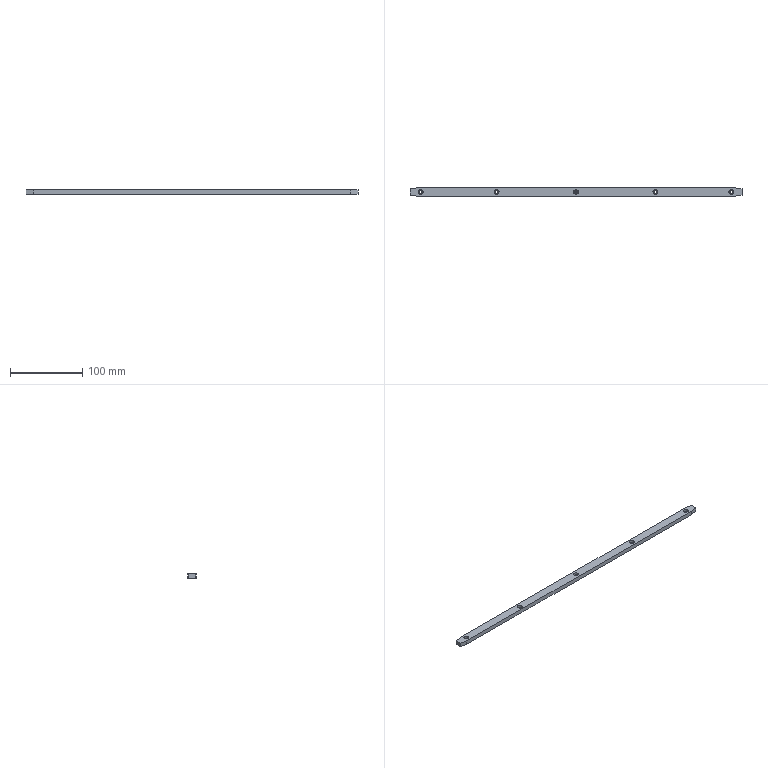Part | NX | features BREP 1 | 1 solid | 35 faces | box 460 x 12 x 6 mm | volume 32178 mm3 | cylinder 20 | plane 15 | commonest cylinder face diameters 3.4 x10 6.7 x10
STEP:
#1=CARTESIAN_POINT('',(-113.35,0.,-0.5));
#2=VERTEX_POINT('',#1);
#3=CARTESIAN_POINT('',(-106.65,0.,-0.5));
#4=VERTEX_POINT('',#3);
#5=CARTESIAN_POINT('',(-110.,0.,-0.5));
#6=DIRECTION('',(0.,0.,1.));
#7=DIRECTION('',(1.,0.,0.));
#8=AXIS2_PLACEMENT_3D('',#5,#6,#7);
#9=CIRCLE('',#8,3.35);
#10=EDGE_CURVE('',#2,#4,#9,.T.);
#11=ORIENTED_EDGE('',*,*,#10,.F.);
#12=CARTESIAN_POINT('',(-113.35,0.,3.));
#13=VERTEX_POINT('',#12);
#14=CARTESIAN_POINT('',(-113.35,0.,3.));
#15=DIRECTION('',(0.,0.,1.));
#16=VECTOR('',#15,1000.);
#17=LINE('',#14,#16);
#18=EDGE_CURVE('',#13,#2,#17,.F.);
#19=ORIENTED_EDGE('',*,*,#18,.F.);
#20=CARTESIAN_POINT('',(-106.65,0.,3.));
#21=VERTEX_POINT('',#20);
#22=CARTESIAN_POINT('',(-110.,0.,3.));
#23=DIRECTION('',(0.,0.,1.));
#24=DIRECTION('',(1.,0.,0.));
#25=AXIS2_PLACEMENT_3D('',#22,#23,#24);
#26=CIRCLE('',#25,3.35);
#27=EDGE_CURVE('',#13,#21,#26,.T.);
#28=ORIENTED_EDGE('',*,*,#27,.T.);
#29=CARTESIAN_POINT('',(-106.65,0.,3.));
#30=DIRECTION('',(0.,0.,1.));
#31=VECTOR('',#30,1000.);
#32=LINE('',#29,#31);
#33=EDGE_CURVE('',#21,#4,#32,.F.);
#34=ORIENTED_EDGE('',*,*,#33,.T.);
#35=EDGE_LOOP('',(#11,#19,#28,#34));
#36=FACE_BOUND('',#35,.T.);
#37=CARTESIAN_POINT('',(-110.,0.,3.));
#38=DIRECTION('',(0.,0.,1.));
#39=DIRECTION('',(1.,0.,0.));
#40=AXIS2_PLACEMENT_3D('',#37,#38,#39);
#41=CYLINDRICAL_SURFACE('',#40,3.35);
#42=ADVANCED_FACE('',(#36),#41,.F.);
#43=CARTESIAN_POINT('',(-111.7,0.,-3.));
#44=VERTEX_POINT('',#43);
#45=CARTESIAN_POINT('',(-108.3,0.,-3.));
#46=VERTEX_POINT('',#45);
#47=CARTESIAN_POINT('',(-110.,0.,-3.));
#48=DIRECTION('',(0.,0.,1.));
#49=DIRECTION('',(1.,0.,0.));
#50=AXIS2_PLACEMENT_3D('',#47,#48,#49);
#51=CIRCLE('',#50,1.7);
#52=EDGE_CURVE('',#44,#46,#51,.T.);
#53=ORIENTED_EDGE('',*,*,#52,.F.);
#54=CARTESIAN_POINT('',(-111.7,0.,-0.5));
#55=VERTEX_POINT('',#54);
#56=CARTESIAN_POINT('',(-111.7,0.,3.));
#57=DIRECTION('',(0.,0.,1.));
#58=VECTOR('',#57,1000.);
#59=LINE('',#56,#58);
#60=EDGE_CURVE('',#55,#44,#59,.F.);
#61=ORIENTED_EDGE('',*,*,#60,.F.);
#62=CARTESIAN_POINT('',(-108.3,0.,-0.5));
#63=VERTEX_POINT('',#62);
#64=CARTESIAN_POINT('',(-110.,0.,-0.5));
#65=DIRECTION('',(0.,0.,1.));
#66=DIRECTION('',(1.,0.,0.));
#67=AXIS2_PLACEMENT_3D('',#64,#65,#66);
#68=CIRCLE('',#67,1.7);
#69=EDGE_CURVE('',#55,#63,#68,.T.);
#70=ORIENTED_EDGE('',*,*,#69,.T.);
#71=CARTESIAN_POINT('',(-108.3,0.,3.));
#72=DIRECTION('',(0.,0.,1.));
#73=VECTOR('',#72,1000.);
#74=LINE('',#71,#73);
#75=EDGE_CURVE('',#63,#46,#74,.F.);
#76=ORIENTED_EDGE('',*,*,#75,.T.);
#77=EDGE_LOOP('',(#53,#61,#70,#76));
#78=FACE_BOUND('',#77,.T.);
#79=CARTESIAN_POINT('',(-110.,0.,3.));
#80=DIRECTION('',(0.,0.,1.));
#81=DIRECTION('',(1.,0.,0.));
#82=AXIS2_PLACEMENT_3D('',#79,#80,#81);
#83=CYLINDRICAL_SURFACE('',#82,1.7);
#84=ADVANCED_FACE('',(#78),#83,.F.);
#85=CARTESIAN_POINT('',(106.65,0.,-0.5));
#86=VERTEX_POINT('',#85);
#87=CARTESIAN_POINT('',(113.35,0.,-0.5));
#88=VERTEX_POINT('',#87);
#89=CARTESIAN_POINT('',(110.,0.,-0.5));
#90=DIRECTION('',(0.,0.,1.));
#91=DIRECTION('',(1.,0.,0.));
#92=AXIS2_PLACEMENT_3D('',#89,#90,#91);
#93=CIRCLE('',#92,3.35);
#94=EDGE_CURVE('',#86,#88,#93,.T.);
#95=ORIENTED_EDGE('',*,*,#94,.F.);
#96=CARTESIAN_POINT('',(106.65,0.,3.));
#97=VERTEX_POINT('',#96);
#98=CARTESIAN_POINT('',(106.65,0.,3.));
#99=DIRECTION('',(0.,0.,1.));
#100=VECTOR('',#99,1000.);
#101=LINE('',#98,#100);
#102=EDGE_CURVE('',#97,#86,#101,.F.);
#103=ORIENTED_EDGE('',*,*,#102,.F.);
#104=CARTESIAN_POINT('',(113.35,0.,3.));
#105=VERTEX_POINT('',#104);
#106=CARTESIAN_POINT('',(110.,0.,3.));
#107=DIRECTION('',(0.,0.,1.));
#108=DIRECTION('',(1.,0.,0.));
#109=AXIS2_PLACEMENT_3D('',#106,#107,#108);
#110=CIRCLE('',#109,3.35);
#111=EDGE_CURVE('',#97,#105,#110,.T.);
#112=ORIENTED_EDGE('',*,*,#111,.T.);
#113=CARTESIAN_POINT('',(113.35,0.,3.));
#114=DIRECTION('',(0.,0.,1.));
#115=VECTOR('',#114,1000.);
#116=LINE('',#113,#115);
#117=EDGE_CURVE('',#105,#88,#116,.F.);
#118=ORIENTED_EDGE('',*,*,#117,.T.);
#119=EDGE_LOOP('',(#95,#103,#112,#118));
#120=FACE_BOUND('',#119,.T.);
#121=CARTESIAN_POINT('',(110.,0.,3.));
#122=DIRECTION('',(0.,0.,1.));
#123=DIRECTION('',(1.,0.,0.));
#124=AXIS2_PLACEMENT_3D('',#121,#122,#123);
#125=CYLINDRICAL_SURFACE('',#124,3.35);
#126=ADVANCED_FACE('',(#120),#125,.F.);
#127=CARTESIAN_POINT('',(108.3,0.,-3.));
#128=VERTEX_POINT('',#127);
#129=CARTESIAN_POINT('',(111.7,0.,-3.));
#130=VERTEX_POINT('',#129);
#131=CARTESIAN_POINT('',(110.,0.,-3.));
#132=DIRECTION('',(0.,0.,1.));
#133=DIRECTION('',(1.,0.,0.));
#134=AXIS2_PLACEMENT_3D('',#131,#132,#133);
#135=CIRCLE('',#134,1.7);
#136=EDGE_CURVE('',#128,#130,#135,.T.);
#137=ORIENTED_EDGE('',*,*,#136,.F.);
#138=CARTESIAN_POINT('',(108.3,0.,-0.5));
#139=VERTEX_POINT('',#138);
#140=CARTESIAN_POINT('',(108.3,0.,3.));
#141=DIRECTION('',(0.,0.,1.));
#142=VECTOR('',#141,1000.);
#143=LINE('',#140,#142);
#144=EDGE_CURVE('',#139,#128,#143,.F.);
#145=ORIENTED_EDGE('',*,*,#144,.F.);
#146=CARTESIAN_POINT('',(111.7,0.,-0.5));
#147=VERTEX_POINT('',#146);
#148=CARTESIAN_POINT('',(110.,0.,-0.5));
#149=DIRECTION('',(0.,0.,1.));
#150=DIRECTION('',(1.,0.,0.));
#151=AXIS2_PLACEMENT_3D('',#148,#149,#150);
#152=CIRCLE('',#151,1.7);
#153=EDGE_CURVE('',#139,#147,#152,.T.);
#154=ORIENTED_EDGE('',*,*,#153,.T.);
#155=CARTESIAN_POINT('',(111.7,0.,3.));
#156=DIRECTION('',(0.,0.,1.));
#157=VECTOR('',#156,1000.);
#158=LINE('',#155,#157);
#159=EDGE_CURVE('',#147,#130,#158,.F.);
#160=ORIENTED_EDGE('',*,*,#159,.T.);
#161=EDGE_LOOP('',(#137,#145,#154,#160));
#162=FACE_BOUND('',#161,.T.);
#163=CARTESIAN_POINT('',(110.,0.,3.));
#164=DIRECTION('',(0.,0.,1.));
#165=DIRECTION('',(1.,0.,0.));
#166=AXIS2_PLACEMENT_3D('',#163,#164,#165);
#167=CYLINDRICAL_SURFACE('',#166,1.7);
#168=ADVANCED_FACE('',(#162),#167,.F.);
#169=CARTESIAN_POINT('',(-3.35,0.,-0.5));
#170=VERTEX_POINT('',#169);
#171=CARTESIAN_POINT('',(3.35,0.,-0.5));
#172=VERTEX_POINT('',#171);
#173=CARTESIAN_POINT('',(0.,0.,-0.5));
#174=DIRECTION('',(0.,0.,1.));
#175=DIRECTION('',(1.,0.,0.));
#176=AXIS2_PLACEMENT_3D('',#173,#174,#175);
#177=CIRCLE('',#176,3.35);
#178=EDGE_CURVE('',#170,#172,#177,.T.);
#179=ORIENTED_EDGE('',*,*,#178,.F.);
#180=CARTESIAN_POINT('',(-3.35,0.,3.));
#181=VERTEX_POINT('',#180);
#182=CARTESIAN_POINT('',(-3.35,0.,3.));
#183=DIRECTION('',(0.,0.,1.));
#184=VECTOR('',#183,1000.);
#185=LINE('',#182,#184);
#186=EDGE_CURVE('',#181,#170,#185,.F.);
#187=ORIENTED_EDGE('',*,*,#186,.F.);
#188=CARTESIAN_POINT('',(3.35,0.,3.));
#189=VERTEX_POINT('',#188);
#190=CARTESIAN_POINT('',(0.,0.,3.));
#191=DIRECTION('',(0.,0.,1.));
#192=DIRECTION('',(1.,0.,0.));
#193=AXIS2_PLACEMENT_3D('',#190,#191,#192);
#194=CIRCLE('',#193,3.35);
#195=EDGE_CURVE('',#181,#189,#194,.T.);
#196=ORIENTED_EDGE('',*,*,#195,.T.);
#197=CARTESIAN_POINT('',(3.35,0.,3.));
#198=DIRECTION('',(0.,0.,1.));
#199=VECTOR('',#198,1000.);
#200=LINE('',#197,#199);
#201=EDGE_CURVE('',#189,#172,#200,.F.);
#202=ORIENTED_EDGE('',*,*,#201,.T.);
#203=EDGE_LOOP('',(#179,#187,#196,#202));
#204=FACE_BOUND('',#203,.T.);
#205=CARTESIAN_POINT('',(0.,0.,3.));
#206=DIRECTION('',(0.,0.,1.));
#207=DIRECTION('',(1.,0.,0.));
#208=AXIS2_PLACEMENT_3D('',#205,#206,#207);
#209=CYLINDRICAL_SURFACE('',#208,3.35);
#210=ADVANCED_FACE('',(#204),#209,.F.);
#211=CARTESIAN_POINT('',(-1.7,0.,-3.));
#212=VERTEX_POINT('',#211);
#213=CARTESIAN_POINT('',(1.7,0.,-3.));
#214=VERTEX_POINT('',#213);
#215=CARTESIAN_POINT('',(0.,0.,-3.));
#216=DIRECTION('',(0.,0.,1.));
#217=DIRECTION('',(1.,0.,0.));
#218=AXIS2_PLACEMENT_3D('',#215,#216,#217);
#219=CIRCLE('',#218,1.7);
#220=EDGE_CURVE('',#212,#214,#219,.T.);
#221=ORIENTED_EDGE('',*,*,#220,.F.);
#222=CARTESIAN_POINT('',(-1.7,0.,-0.5));
#223=VERTEX_POINT('',#222);
#224=CARTESIAN_POINT('',(-1.7,0.,3.));
#225=DIRECTION('',(0.,0.,1.));
#226=VECTOR('',#225,1000.);
#227=LINE('',#224,#226);
#228=EDGE_CURVE('',#223,#212,#227,.F.);
#229=ORIENTED_EDGE('',*,*,#228,.F.);
#230=CARTESIAN_POINT('',(1.7,0.,-0.5));
#231=VERTEX_POINT('',#230);
#232=CARTESIAN_POINT('',(0.,0.,-0.5));
#233=DIRECTION('',(0.,0.,1.));
#234=DIRECTION('',(1.,0.,0.));
#235=AXIS2_PLACEMENT_3D('',#232,#233,#234);
#236=CIRCLE('',#235,1.7);
#237=EDGE_CURVE('',#223,#231,#236,.T.);
#238=ORIENTED_EDGE('',*,*,#237,.T.);
#239=CARTESIAN_POINT('',(1.7,0.,3.));
#240=DIRECTION('',(0.,0.,1.));
#241=VECTOR('',#240,1000.);
#242=LINE('',#239,#241);
#243=EDGE_CURVE('',#231,#214,#242,.F.);
#244=ORIENTED_EDGE('',*,*,#243,.T.);
#245=EDGE_LOOP('',(#221,#229,#238,#244));
#246=FACE_BOUND('',#245,.T.);
#247=CARTESIAN_POINT('',(0.,0.,3.));
#248=DIRECTION('',(0.,0.,1.));
#249=DIRECTION('',(1.,0.,0.));
#250=AXIS2_PLACEMENT_3D('',#247,#248,#249);
#251=CYLINDRICAL_SURFACE('',#250,1.7);
#252=ADVANCED_FACE('',(#246),#251,.F.);
#253=CARTESIAN_POINT('',(-218.35,0.,-0.5));
#254=VERTEX_POINT('',#253);
#255=CARTESIAN_POINT('',(-211.65,0.,-0.5));
#256=VERTEX_POINT('',#255);
#257=CARTESIAN_POINT('',(-215.,0.,-0.5));
#258=DIRECTION('',(0.,0.,1.));
#259=DIRECTION('',(1.,0.,0.));
#260=AXIS2_PLACEMENT_3D('',#257,#258,#259);
#261=CIRCLE('',#260,3.35);
#262=EDGE_CURVE('',#254,#256,#261,.T.);
#263=ORIENTED_EDGE('',*,*,#262,.F.);
#264=CARTESIAN_POINT('',(-218.35,0.,3.));
#265=VERTEX_POINT('',#264);
#266=CARTESIAN_POINT('',(-218.35,0.,3.));
#267=DIRECTION('',(0.,0.,1.));
#268=VECTOR('',#267,1000.);
#269=LINE('',#266,#268);
#270=EDGE_CURVE('',#265,#254,#269,.F.);
#271=ORIENTED_EDGE('',*,*,#270,.F.);
#272=CARTESIAN_POINT('',(-211.65,0.,3.));
#273=VERTEX_POINT('',#272);
#274=CARTESIAN_POINT('',(-215.,0.,3.));
#275=DIRECTION('',(0.,0.,1.));
#276=DIRECTION('',(1.,0.,0.));
#277=AXIS2_PLACEMENT_3D('',#274,#275,#276);
#278=CIRCLE('',#277,3.35);
#279=EDGE_CURVE('',#265,#273,#278,.T.);
#280=ORIENTED_EDGE('',*,*,#279,.T.);
#281=CARTESIAN_POINT('',(-211.65,0.,3.));
#282=DIRECTION('',(0.,0.,1.));
#283=VECTOR('',#282,1000.);
#284=LINE('',#281,#283);
#285=EDGE_CURVE('',#273,#256,#284,.F.);
#286=ORIENTED_EDGE('',*,*,#285,.T.);
#287=EDGE_LOOP('',(#263,#271,#280,#286));
#288=FACE_BOUND('',#287,.T.);
#289=CARTESIAN_POINT('',(-215.,0.,3.));
#290=DIRECTION('',(0.,0.,1.));
#291=DIRECTION('',(1.,0.,0.));
#292=AXIS2_PLACEMENT_3D('',#289,#290,#291);
#293=CYLINDRICAL_SURFACE('',#292,3.35);
#294=ADVANCED_FACE('',(#288),#293,.F.);
#295=CARTESIAN_POINT('',(-216.7,0.,-3.));
#296=VERTEX_POINT('',#295);
#297=CARTESIAN_POINT('',(-213.3,0.,-3.));
#298=VERTEX_POINT('',#297);
#299=CARTESIAN_POINT('',(-215.,0.,-3.));
#300=DIRECTION('',(0.,0.,1.));
#301=DIRECTION('',(1.,0.,0.));
#302=AXIS2_PLACEMENT_3D('',#299,#300,#301);
#303=CIRCLE('',#302,1.7);
#304=EDGE_CURVE('',#296,#298,#303,.T.);
#305=ORIENTED_EDGE('',*,*,#304,.F.);
#306=CARTESIAN_POINT('',(-216.7,0.,-0.5));
#307=VERTEX_POINT('',#306);
#308=CARTESIAN_POINT('',(-216.7,0.,3.));
#309=DIRECTION('',(0.,0.,1.));
#310=VECTOR('',#309,1000.);
#311=LINE('',#308,#310);
#312=EDGE_CURVE('',#307,#296,#311,.F.);
#313=ORIENTED_EDGE('',*,*,#312,.F.);
#314=CARTESIAN_POINT('',(-213.3,0.,-0.5));
#315=VERTEX_POINT('',#314);
#316=CARTESIAN_POINT('',(-215.,0.,-0.5));
#317=DIRECTION('',(0.,0.,1.));
#318=DIRECTION('',(1.,0.,0.));
#319=AXIS2_PLACEMENT_3D('',#316,#317,#318);
#320=CIRCLE('',#319,1.7);
#321=EDGE_CURVE('',#307,#315,#320,.T.);
#322=ORIENTED_EDGE('',*,*,#321,.T.);
#323=CARTESIAN_POINT('',(-213.3,0.,3.));
#324=DIRECTION('',(0.,0.,1.));
#325=VECTOR('',#324,1000.);
#326=LINE('',#323,#325);
#327=EDGE_CURVE('',#315,#298,#326,.F.);
#328=ORIENTED_EDGE('',*,*,#327,.T.);
#329=EDGE_LOOP('',(#305,#313,#322,#328));
#330=FACE_BOUND('',#329,.T.);
#331=CARTESIAN_POINT('',(-215.,0.,3.));
#332=DIRECTION('',(0.,0.,1.));
#333=DIRECTION('',(1.,0.,0.));
#334=AXIS2_PLACEMENT_3D('',#331,#332,#333);
#335=CYLINDRICAL_SURFACE('',#334,1.7);
#336=ADVANCED_FACE('',(#330),#335,.F.);
#337=CARTESIAN_POINT('',(211.65,0.,-0.5));
#338=VERTEX_POINT('',#337);
#339=CARTESIAN_POINT('',(218.35,0.,-0.5));
#340=VERTEX_POINT('',#339);
#341=CARTESIAN_POINT('',(215.,0.,-0.5));
#342=DIRECTION('',(0.,0.,1.));
#343=DIRECTION('',(1.,0.,0.));
#344=AXIS2_PLACEMENT_3D('',#341,#342,#343);
#345=CIRCLE('',#344,3.35);
#346=EDGE_CURVE('',#338,#340,#345,.T.);
#347=ORIENTED_EDGE('',*,*,#346,.F.);
#348=CARTESIAN_POINT('',(211.65,0.,3.));
#349=VERTEX_POINT('',#348);
#350=CARTESIAN_POINT('',(211.65,0.,3.));
#351=DIRECTION('',(0.,0.,1.));
#352=VECTOR('',#351,1000.);
#353=LINE('',#350,#352);
#354=EDGE_CURVE('',#349,#338,#353,.F.);
#355=ORIENTED_EDGE('',*,*,#354,.F.);
#356=CARTESIAN_POINT('',(218.35,0.,3.));
#357=VERTEX_POINT('',#356);
#358=CARTESIAN_POINT('',(215.,0.,3.));
#359=DIRECTION('',(0.,0.,1.));
#360=DIRECTION('',(1.,0.,0.));
#361=AXIS2_PLACEMENT_3D('',#358,#359,#360);
#362=CIRCLE('',#361,3.35);
#363=EDGE_CURVE('',#349,#357,#362,.T.);
#364=ORIENTED_EDGE('',*,*,#363,.T.);
#365=CARTESIAN_POINT('',(218.35,0.,3.));
#366=DIRECTION('',(0.,0.,1.));
#367=VECTOR('',#366,1000.);
#368=LINE('',#365,#367);
#369=EDGE_CURVE('',#357,#340,#368,.F.);
#370=ORIENTED_EDGE('',*,*,#369,.T.);
#371=EDGE_LOOP('',(#347,#355,#364,#370));
#372=FACE_BOUND('',#371,.T.);
#373=CARTESIAN_POINT('',(215.,0.,3.));
#374=DIRECTION('',(0.,0.,1.));
#375=DIRECTION('',(1.,0.,0.));
#376=AXIS2_PLACEMENT_3D('',#373,#374,#375);
#377=CYLINDRICAL_SURFACE('',#376,3.35);
#378=ADVANCED_FACE('',(#372),#377,.F.);
#379=CARTESIAN_POINT('',(213.3,0.,-3.));
#380=VERTEX_POINT('',#379);
#381=CARTESIAN_POINT('',(216.7,0.,-3.));
#382=VERTEX_POINT('',#381);
#383=CARTESIAN_POINT('',(215.,0.,-3.));
#384=DIRECTION('',(0.,0.,1.));
#385=DIRECTION('',(1.,0.,0.));
#386=AXIS2_PLACEMENT_3D('',#383,#384,#385);
#387=CIRCLE('',#386,1.7);
#388=EDGE_CURVE('',#380,#382,#387,.T.);
#389=ORIENTED_EDGE('',*,*,#388,.F.);
#390=CARTESIAN_POINT('',(213.3,0.,-0.5));
#391=VERTEX_POINT('',#390);
#392=CARTESIAN_POINT('',(213.3,0.,3.));
#393=DIRECTION('',(0.,0.,1.));
#394=VECTOR('',#393,1000.);
#395=LINE('',#392,#394);
#396=EDGE_CURVE('',#391,#380,#395,.F.);
#397=ORIENTED_EDGE('',*,*,#396,.F.);
#398=CARTESIAN_POINT('',(216.7,0.,-0.5));
#399=VERTEX_POINT('',#398);
#400=CARTESIAN_POINT('',(215.,0.,-0.5));
#401=DIRECTION('',(0.,0.,1.));
#402=DIRECTION('',(1.,0.,0.));
#403=AXIS2_PLACEMENT_3D('',#400,#401,#402);
#404=CIRCLE('',#403,1.7);
#405=EDGE_CURVE('',#391,#399,#404,.T.);
#406=ORIENTED_EDGE('',*,*,#405,.T.);
#407=CARTESIAN_POINT('',(216.7,0.,3.));
#408=DIRECTION('',(0.,0.,1.));
#409=VECTOR('',#408,1000.);
#410=LINE('',#407,#409);
#411=EDGE_CURVE('',#399,#382,#410,.F.);
#412=ORIENTED_EDGE('',*,*,#411,.T.);
#413=EDGE_LOOP('',(#389,#397,#406,#412));
#414=FACE_BOUND('',#413,.T.);
#415=CARTESIAN_POINT('',(215.,0.,3.));
#416=DIRECTION('',(0.,0.,1.));
#417=DIRECTION('',(1.,0.,0.));
#418=AXIS2_PLACEMENT_3D('',#415,#416,#417);
#419=CYLINDRICAL_SURFACE('',#418,1.7);
#420=ADVANCED_FACE('',(#414),#419,.F.);
#421=CARTESIAN_POINT('',(230.,-4.237,3.));
#422=VERTEX_POINT('',#421);
#423=CARTESIAN_POINT('',(230.,4.237,3.));
#424=VERTEX_POINT('',#423);
#425=CARTESIAN_POINT('',(230.,-6.,3.));
#426=DIRECTION('',(0.,1.,0.));
#427=VECTOR('',#426,1000.);
#428=LINE('',#425,#427);
#429=EDGE_CURVE('',#422,#424,#428,.T.);
#430=ORIENTED_EDGE('',*,*,#429,.F.);
#431=CARTESIAN_POINT('',(230.,-4.237,-3.));
#432=VERTEX_POINT('',#431);
#433=CARTESIAN_POINT('',(230.,-4.237,3.));
#434=DIRECTION('',(0.,0.,-1.));
#435=VECTOR('',#434,1000.);
#436=LINE('',#433,#435);
#437=EDGE_CURVE('',#422,#432,#436,.T.);
#438=ORIENTED_EDGE('',*,*,#437,.T.);
#439=CARTESIAN_POINT('',(230.,4.237,-3.));
#440=VERTEX_POINT('',#439);
#441=CARTESIAN_POINT('',(230.,-6.,-3.));
#442=DIRECTION('',(0.,1.,0.));
#443=VECTOR('',#442,1000.);
#444=LINE('',#441,#443);
#445=EDGE_CURVE('',#432,#440,#444,.T.);
#446=ORIENTED_EDGE('',*,*,#445,.T.);
#447=CARTESIAN_POINT('',(230.,4.237,3.));
#448=DIRECTION('',(0.,0.,1.));
#449=VECTOR('',#448,1000.);
#450=LINE('',#447,#449);
#451=EDGE_CURVE('',#440,#424,#450,.T.);
#452=ORIENTED_EDGE('',*,*,#451,.T.);
#453=EDGE_LOOP('',(#430,#438,#446,#452));
#454=FACE_BOUND('',#453,.T.);
#455=CARTESIAN_POINT('',(230.,-6.,3.));
#456=DIRECTION('',(-1.,0.,0.));
#457=DIRECTION('',(0.,0.,1.));
#458=AXIS2_PLACEMENT_3D('',#455,#456,#457);
#459=PLANE('',#458);
#460=ADVANCED_FACE('',(#454),#459,.F.);
#461=CARTESIAN_POINT('',(220.,6.,3.));
#462=VERTEX_POINT('',#461);
#463=CARTESIAN_POINT('',(-220.,6.,3.));
#464=VERTEX_POINT('',#463);
#465=CARTESIAN_POINT('',(-230.,6.,3.));
#466=DIRECTION('',(-1.,0.,0.));
#467=VECTOR('',#466,1000.);
#468=LINE('',#465,#467);
#469=EDGE_CURVE('',#462,#464,#468,.T.);
#470=ORIENTED_EDGE('',*,*,#469,.F.);
#471=CARTESIAN_POINT('',(220.,6.,-3.));
#472=VERTEX_POINT('',#471);
#473=CARTESIAN_POINT('',(220.,6.,3.));
#474=DIRECTION('',(0.,0.,-1.));
#475=VECTOR('',#474,1000.);
#476=LINE('',#473,#475);
#477=EDGE_CURVE('',#462,#472,#476,.T.);
#478=ORIENTED_EDGE('',*,*,#477,.T.);
#479=CARTESIAN_POINT('',(-220.,6.,-3.));
#480=VERTEX_POINT('',#479);
#481=CARTESIAN_POINT('',(-230.,6.,-3.));
#482=DIRECTION('',(-1.,0.,0.));
#483=VECTOR('',#482,1000.);
#484=LINE('',#481,#483);
#485=EDGE_CURVE('',#472,#480,#484,.T.);
#486=ORIENTED_EDGE('',*,*,#485,.T.);
#487=CARTESIAN_POINT('',(-220.,6.,3.));
#488=DIRECTION('',(0.,0.,1.));
#489=VECTOR('',#488,1000.);
#490=LINE('',#487,#489);
#491=EDGE_CURVE('',#480,#464,#490,.T.);
#492=ORIENTED_EDGE('',*,*,#491,.T.);
#493=EDGE_LOOP('',(#470,#478,#486,#492));
#494=FACE_BOUND('',#493,.T.);
#495=CARTESIAN_POINT('',(-230.,6.,3.));
#496=DIRECTION('',(0.,-1.,0.));
#497=DIRECTION('',(0.,0.,-1.));
#498=AXIS2_PLACEMENT_3D('',#495,#496,#497);
#499=PLANE('',#498);
#500=ADVANCED_FACE('',(#494),#499,.F.);
#501=CARTESIAN_POINT('',(-230.,4.237,-3.));
#502=VERTEX_POINT('',#501);
#503=CARTESIAN_POINT('',(-230.,-4.237,-3.));
#504=VERTEX_POINT('',#503);
#505=CARTESIAN_POINT('',(-230.,-6.,-3.));
#506=DIRECTION('',(0.,-1.,0.));
#507=VECTOR('',#506,1000.);
#508=LINE('',#505,#507);
#509=EDGE_CURVE('',#502,#504,#508,.T.);
#510=ORIENTED_EDGE('',*,*,#509,.T.);
#511=CARTESIAN_POINT('',(-230.,-4.237,3.));
#512=VERTEX_POINT('',#511);
#513=CARTESIAN_POINT('',(-230.,-4.237,3.));
#514=DIRECTION('',(0.,0.,1.));
#515=VECTOR('',#514,1000.);
#516=LINE('',#513,#515);
#517=EDGE_CURVE('',#504,#512,#516,.T.);
#518=ORIENTED_EDGE('',*,*,#517,.T.);
#519=CARTESIAN_POINT('',(-230.,4.237,3.));
#520=VERTEX_POINT('',#519);
#521=CARTESIAN_POINT('',(-230.,-6.,3.));
#522=DIRECTION('',(0.,-1.,0.));
#523=VECTOR('',#522,1000.);
#524=LINE('',#521,#523);
#525=EDGE_CURVE('',#520,#512,#524,.T.);
#526=ORIENTED_EDGE('',*,*,#525,.F.);
#527=CARTESIAN_POINT('',(-230.,4.237,3.));
#528=DIRECTION('',(0.,0.,-1.));
#529=VECTOR('',#528,1000.);
#530=LINE('',#527,#529);
#531=EDGE_CURVE('',#520,#502,#530,.T.);
#532=ORIENTED_EDGE('',*,*,#531,.T.);
#533=EDGE_LOOP('',(#510,#518,#526,#532));
#534=FACE_BOUND('',#533,.T.);
#535=CARTESIAN_POINT('',(-230.,-6.,3.));
#536=DIRECTION('',(1.,0.,0.));
#537=DIRECTION('',(0.,1.,0.));
#538=AXIS2_PLACEMENT_3D('',#535,#536,#537);
#539=PLANE('',#538);
#540=ADVANCED_FACE('',(#534),#539,.F.);
#541=CARTESIAN_POINT('',(-220.,-6.,-3.));
#542=VERTEX_POINT('',#541);
#543=CARTESIAN_POINT('',(220.,-6.,-3.));
#544=VERTEX_POINT('',#543);
#545=CARTESIAN_POINT('',(-230.,-6.,-3.));
#546=DIRECTION('',(1.,0.,0.));
#547=VECTOR('',#546,1000.);
#548=LINE('',#545,#547);
#549=EDGE_CURVE('',#542,#544,#548,.T.);
#550=ORIENTED_EDGE('',*,*,#549,.T.);
#551=CARTESIAN_POINT('',(220.,-6.,3.));
#552=VERTEX_POINT('',#551);
#553=CARTESIAN_POINT('',(220.,-6.,3.));
#554=DIRECTION('',(0.,0.,1.));
#555=VECTOR('',#554,1000.);
#556=LINE('',#553,#555);
#557=EDGE_CURVE('',#544,#552,#556,.T.);
#558=ORIENTED_EDGE('',*,*,#557,.T.);
#559=CARTESIAN_POINT('',(-220.,-6.,3.));
#560=VERTEX_POINT('',#559);
#561=CARTESIAN_POINT('',(-230.,-6.,3.));
#562=DIRECTION('',(1.,0.,0.));
#563=VECTOR('',#562,1000.);
#564=LINE('',#561,#563);
#565=EDGE_CURVE('',#560,#552,#564,.T.);
#566=ORIENTED_EDGE('',*,*,#565,.F.);
#567=CARTESIAN_POINT('',(-220.,-6.,3.));
#568=DIRECTION('',(0.,0.,-1.));
#569=VECTOR('',#568,1000.);
#570=LINE('',#567,#569);
#571=EDGE_CURVE('',#560,#542,#570,.T.);
#572=ORIENTED_EDGE('',*,*,#571,.T.);
#573=EDGE_LOOP('',(#550,#558,#566,#572));
#574=FACE_BOUND('',#573,.T.);
#575=CARTESIAN_POINT('',(-230.,-6.,3.));
#576=DIRECTION('',(0.,1.,0.));
#577=DIRECTION('',(1.,0.,0.));
#578=AXIS2_PLACEMENT_3D('',#575,#576,#577);
#579=PLANE('',#578);
#580=ADVANCED_FACE('',(#574),#579,.F.);
#581=ORIENTED_EDGE('',*,*,#565,.T.);
#582=CARTESIAN_POINT('',(230.,-4.237,3.));
#583=DIRECTION('',(0.9848,0.1736,0.));
#584=VECTOR('',#583,1000.);
#585=LINE('',#582,#584);
#586=EDGE_CURVE('',#552,#422,#585,.T.);
#587=ORIENTED_EDGE('',*,*,#586,.T.);
#588=ORIENTED_EDGE('',*,*,#429,.T.);
#589=CARTESIAN_POINT('',(220.,6.,3.));
#590=DIRECTION('',(-0.9848,0.1736,0.));
#591=VECTOR('',#590,1000.);
#592=LINE('',#589,#591);
#593=EDGE_CURVE('',#424,#462,#592,.T.);
#594=ORIENTED_EDGE('',*,*,#593,.T.);
#595=ORIENTED_EDGE('',*,*,#469,.T.);
#596=CARTESIAN_POINT('',(-230.,4.237,3.));
#597=DIRECTION('',(-0.9848,-0.1736,0.));
#598=VECTOR('',#597,1000.);
#599=LINE('',#596,#598);
#600=EDGE_CURVE('',#464,#520,#599,.T.);
#601=ORIENTED_EDGE('',*,*,#600,.T.);
#602=ORIENTED_EDGE('',*,*,#525,.T.);
#603=CARTESIAN_POINT('',(-220.,-6.,3.));
#604=DIRECTION('',(0.9848,-0.1736,0.));
#605=VECTOR('',#604,1000.);
#606=LINE('',#603,#605);
#607=EDGE_CURVE('',#512,#560,#606,.T.);
#608=ORIENTED_EDGE('',*,*,#607,.T.);
#609=EDGE_LOOP('',(#581,#587,#588,#594,#595,#601,#602,#608));
#610=FACE_BOUND('',#609,.T.);
#611=CARTESIAN_POINT('',(-110.,0.,3.));
#612=DIRECTION('',(0.,0.,1.));
#613=DIRECTION('',(1.,0.,0.));
#614=AXIS2_PLACEMENT_3D('',#611,#612,#613);
#615=CIRCLE('',#614,3.35);
#616=EDGE_CURVE('',#21,#13,#615,.T.);
#617=ORIENTED_EDGE('',*,*,#616,.F.);
#618=ORIENTED_EDGE('',*,*,#27,.F.);
#619=EDGE_LOOP('',(#617,#618));
#620=FACE_BOUND('',#619,.T.);
#621=CARTESIAN_POINT('',(110.,0.,3.));
#622=DIRECTION('',(0.,0.,1.));
#623=DIRECTION('',(1.,0.,0.));
#624=AXIS2_PLACEMENT_3D('',#621,#622,#623);
#625=CIRCLE('',#624,3.35);
#626=EDGE_CURVE('',#105,#97,#625,.T.);
#627=ORIENTED_EDGE('',*,*,#626,.F.);
#628=ORIENTED_EDGE('',*,*,#111,.F.);
#629=EDGE_LOOP('',(#627,#628));
#630=FACE_BOUND('',#629,.T.);
#631=CARTESIAN_POINT('',(0.,0.,3.));
#632=DIRECTION('',(0.,0.,1.));
#633=DIRECTION('',(1.,0.,0.));
#634=AXIS2_PLACEMENT_3D('',#631,#632,#633);
#635=CIRCLE('',#634,3.35);
#636=EDGE_CURVE('',#189,#181,#635,.T.);
#637=ORIENTED_EDGE('',*,*,#636,.F.);
#638=ORIENTED_EDGE('',*,*,#195,.F.);
#639=EDGE_LOOP('',(#637,#638));
#640=FACE_BOUND('',#639,.T.);
#641=CARTESIAN_POINT('',(-215.,0.,3.));
#642=DIRECTION('',(0.,0.,1.));
#643=DIRECTION('',(1.,0.,0.));
#644=AXIS2_PLACEMENT_3D('',#641,#642,#643);
#645=CIRCLE('',#644,3.35);
#646=EDGE_CURVE('',#273,#265,#645,.T.);
#647=ORIENTED_EDGE('',*,*,#646,.F.);
#648=ORIENTED_EDGE('',*,*,#279,.F.);
#649=EDGE_LOOP('',(#647,#648));
#650=FACE_BOUND('',#649,.T.);
#651=CARTESIAN_POINT('',(215.,0.,3.));
#652=DIRECTION('',(0.,0.,1.));
#653=DIRECTION('',(1.,0.,0.));
#654=AXIS2_PLACEMENT_3D('',#651,#652,#653);
#655=CIRCLE('',#654,3.35);
#656=EDGE_CURVE('',#357,#349,#655,.T.);
#657=ORIENTED_EDGE('',*,*,#656,.F.);
#658=ORIENTED_EDGE('',*,*,#363,.F.);
#659=EDGE_LOOP('',(#657,#658));
#660=FACE_BOUND('',#659,.T.);
#661=CARTESIAN_POINT('',(0.,0.,3.));
#662=DIRECTION('',(0.,0.,-1.));
#663=DIRECTION('',(0.,-1.,0.));
#664=AXIS2_PLACEMENT_3D('',#661,#662,#663);
#665=PLANE('',#664);
#666=ADVANCED_FACE('',(#610,#620,#630,#640,#650,#660),#665,.F.);
#667=ORIENTED_EDGE('',*,*,#445,.F.);
#668=CARTESIAN_POINT('',(7.66,-43.441,-3.));
#669=DIRECTION('',(-0.9848,-0.1736,0.));
#670=VECTOR('',#669,1000.);
#671=LINE('',#668,#670);
#672=EDGE_CURVE('',#432,#544,#671,.T.);
#673=ORIENTED_EDGE('',*,*,#672,.T.);
#674=ORIENTED_EDGE('',*,*,#549,.F.);
#675=CARTESIAN_POINT('',(-7.66,-43.441,-3.));
#676=DIRECTION('',(-0.9848,0.1736,0.));
#677=VECTOR('',#676,1000.);
#678=LINE('',#675,#677);
#679=EDGE_CURVE('',#542,#504,#678,.T.);
#680=ORIENTED_EDGE('',*,*,#679,.T.);
#681=ORIENTED_EDGE('',*,*,#509,.F.);
#682=CARTESIAN_POINT('',(-7.66,43.441,-3.));
#683=DIRECTION('',(0.9848,0.1736,0.));
#684=VECTOR('',#683,1000.);
#685=LINE('',#682,#684);
#686=EDGE_CURVE('',#502,#480,#685,.T.);
#687=ORIENTED_EDGE('',*,*,#686,.T.);
#688=ORIENTED_EDGE('',*,*,#485,.F.);
#689=CARTESIAN_POINT('',(7.66,43.441,-3.));
#690=DIRECTION('',(0.9848,-0.1736,0.));
#691=VECTOR('',#690,1000.);
#692=LINE('',#689,#691);
#693=EDGE_CURVE('',#472,#440,#692,.T.);
#694=ORIENTED_EDGE('',*,*,#693,.T.);
#695=EDGE_LOOP('',(#667,#673,#674,#680,#681,#687,#688,#694));
#696=FACE_BOUND('',#695,.T.);
#697=CARTESIAN_POINT('',(-110.,0.,-3.));
#698=DIRECTION('',(0.,0.,1.));
#699=DIRECTION('',(1.,0.,0.));
#700=AXIS2_PLACEMENT_3D('',#697,#698,#699);
#701=CIRCLE('',#700,1.7);
#702=EDGE_CURVE('',#46,#44,#701,.T.);
#703=ORIENTED_EDGE('',*,*,#702,.T.);
#704=ORIENTED_EDGE('',*,*,#52,.T.);
#705=EDGE_LOOP('',(#703,#704));
#706=FACE_BOUND('',#705,.T.);
#707=CARTESIAN_POINT('',(110.,0.,-3.));
#708=DIRECTION('',(0.,0.,1.));
#709=DIRECTION('',(1.,0.,0.));
#710=AXIS2_PLACEMENT_3D('',#707,#708,#709);
#711=CIRCLE('',#710,1.7);
#712=EDGE_CURVE('',#130,#128,#711,.T.);
#713=ORIENTED_EDGE('',*,*,#712,.T.);
#714=ORIENTED_EDGE('',*,*,#136,.T.);
#715=EDGE_LOOP('',(#713,#714));
#716=FACE_BOUND('',#715,.T.);
#717=CARTESIAN_POINT('',(0.,0.,-3.));
#718=DIRECTION('',(0.,0.,1.));
#719=DIRECTION('',(1.,0.,0.));
#720=AXIS2_PLACEMENT_3D('',#717,#718,#719);
#721=CIRCLE('',#720,1.7);
#722=EDGE_CURVE('',#214,#212,#721,.T.);
#723=ORIENTED_EDGE('',*,*,#722,.T.);
#724=ORIENTED_EDGE('',*,*,#220,.T.);
#725=EDGE_LOOP('',(#723,#724));
#726=FACE_BOUND('',#725,.T.);
#727=CARTESIAN_POINT('',(-215.,0.,-3.));
#728=DIRECTION('',(0.,0.,1.));
#729=DIRECTION('',(1.,0.,0.));
#730=AXIS2_PLACEMENT_3D('',#727,#728,#729);
#731=CIRCLE('',#730,1.7);
#732=EDGE_CURVE('',#298,#296,#731,.T.);
#733=ORIENTED_EDGE('',*,*,#732,.T.);
#734=ORIENTED_EDGE('',*,*,#304,.T.);
#735=EDGE_LOOP('',(#733,#734));
#736=FACE_BOUND('',#735,.T.);
#737=CARTESIAN_POINT('',(215.,0.,-3.));
#738=DIRECTION('',(0.,0.,1.));
#739=DIRECTION('',(1.,0.,0.));
#740=AXIS2_PLACEMENT_3D('',#737,#738,#739);
#741=CIRCLE('',#740,1.7);
#742=EDGE_CURVE('',#382,#380,#741,.T.);
#743=ORIENTED_EDGE('',*,*,#742,.T.);
#744=ORIENTED_EDGE('',*,*,#388,.T.);
#745=EDGE_LOOP('',(#743,#744));
#746=FACE_BOUND('',#745,.T.);
#747=CARTESIAN_POINT('',(0.,0.,-3.));
#748=DIRECTION('',(0.,0.,-1.));
#749=DIRECTION('',(0.,-1.,0.));
#750=AXIS2_PLACEMENT_3D('',#747,#748,#749);
#751=PLANE('',#750);
#752=ADVANCED_FACE('',(#696,#706,#716,#726,#736,#746),#751,.T.);
#753=ORIENTED_EDGE('',*,*,#396,.T.);
#754=ORIENTED_EDGE('',*,*,#742,.F.);
#755=ORIENTED_EDGE('',*,*,#411,.F.);
#756=CARTESIAN_POINT('',(215.,0.,-0.5));
#757=DIRECTION('',(0.,0.,1.));
#758=DIRECTION('',(1.,0.,0.));
#759=AXIS2_PLACEMENT_3D('',#756,#757,#758);
#760=CIRCLE('',#759,1.7);
#761=EDGE_CURVE('',#399,#391,#760,.T.);
#762=ORIENTED_EDGE('',*,*,#761,.T.);
#763=EDGE_LOOP('',(#753,#754,#755,#762));
#764=FACE_BOUND('',#763,.T.);
#765=CARTESIAN_POINT('',(215.,0.,3.));
#766=DIRECTION('',(0.,0.,1.));
#767=DIRECTION('',(1.,0.,0.));
#768=AXIS2_PLACEMENT_3D('',#765,#766,#767);
#769=CYLINDRICAL_SURFACE('',#768,1.7);
#770=ADVANCED_FACE('',(#764),#769,.F.);
#771=CARTESIAN_POINT('',(215.,0.,-0.5));
#772=DIRECTION('',(0.,0.,1.));
#773=DIRECTION('',(1.,0.,0.));
#774=AXIS2_PLACEMENT_3D('',#771,#772,#773);
#775=CIRCLE('',#774,3.35);
#776=EDGE_CURVE('',#340,#338,#775,.T.);
#777=ORIENTED_EDGE('',*,*,#776,.T.);
#778=ORIENTED_EDGE('',*,*,#346,.T.);
#779=EDGE_LOOP('',(#777,#778));
#780=FACE_BOUND('',#779,.T.);
#781=ORIENTED_EDGE('',*,*,#761,.F.);
#782=ORIENTED_EDGE('',*,*,#405,.F.);
#783=EDGE_LOOP('',(#781,#782));
#784=FACE_BOUND('',#783,.T.);
#785=CARTESIAN_POINT('',(216.7,0.,-0.5));
#786=DIRECTION('',(0.,0.,-1.));
#787=DIRECTION('',(0.,-1.,0.));
#788=AXIS2_PLACEMENT_3D('',#785,#786,#787);
#789=PLANE('',#788);
#790=ADVANCED_FACE('',(#780,#784),#789,.F.);
#791=ORIENTED_EDGE('',*,*,#354,.T.);
#792=ORIENTED_EDGE('',*,*,#776,.F.);
#793=ORIENTED_EDGE('',*,*,#369,.F.);
#794=ORIENTED_EDGE('',*,*,#656,.T.);
#795=EDGE_LOOP('',(#791,#792,#793,#794));
#796=FACE_BOUND('',#795,.T.);
#797=CARTESIAN_POINT('',(215.,0.,3.));
#798=DIRECTION('',(0.,0.,1.));
#799=DIRECTION('',(1.,0.,0.));
#800=AXIS2_PLACEMENT_3D('',#797,#798,#799);
#801=CYLINDRICAL_SURFACE('',#800,3.35);
#802=ADVANCED_FACE('',(#796),#801,.F.);
#803=ORIENTED_EDGE('',*,*,#312,.T.);
#804=ORIENTED_EDGE('',*,*,#732,.F.);
#805=ORIENTED_EDGE('',*,*,#327,.F.);
#806=CARTESIAN_POINT('',(-215.,0.,-0.5));
#807=DIRECTION('',(0.,0.,1.));
#808=DIRECTION('',(1.,0.,0.));
#809=AXIS2_PLACEMENT_3D('',#806,#807,#808);
#810=CIRCLE('',#809,1.7);
#811=EDGE_CURVE('',#315,#307,#810,.T.);
#812=ORIENTED_EDGE('',*,*,#811,.T.);
#813=EDGE_LOOP('',(#803,#804,#805,#812));
#814=FACE_BOUND('',#813,.T.);
#815=CARTESIAN_POINT('',(-215.,0.,3.));
#816=DIRECTION('',(0.,0.,1.));
#817=DIRECTION('',(1.,0.,0.));
#818=AXIS2_PLACEMENT_3D('',#815,#816,#817);
#819=CYLINDRICAL_SURFACE('',#818,1.7);
#820=ADVANCED_FACE('',(#814),#819,.F.);
#821=CARTESIAN_POINT('',(-215.,0.,-0.5));
#822=DIRECTION('',(0.,0.,1.));
#823=DIRECTION('',(1.,0.,0.));
#824=AXIS2_PLACEMENT_3D('',#821,#822,#823);
#825=CIRCLE('',#824,3.35);
#826=EDGE_CURVE('',#256,#254,#825,.T.);
#827=ORIENTED_EDGE('',*,*,#826,.T.);
#828=ORIENTED_EDGE('',*,*,#262,.T.);
#829=EDGE_LOOP('',(#827,#828));
#830=FACE_BOUND('',#829,.T.);
#831=ORIENTED_EDGE('',*,*,#811,.F.);
#832=ORIENTED_EDGE('',*,*,#321,.F.);
#833=EDGE_LOOP('',(#831,#832));
#834=FACE_BOUND('',#833,.T.);
#835=CARTESIAN_POINT('',(-213.3,0.,-0.5));
#836=DIRECTION('',(0.,0.,-1.));
#837=DIRECTION('',(0.,-1.,0.));
#838=AXIS2_PLACEMENT_3D('',#835,#836,#837);
#839=PLANE('',#838);
#840=ADVANCED_FACE('',(#830,#834),#839,.F.);
#841=ORIENTED_EDGE('',*,*,#270,.T.);
#842=ORIENTED_EDGE('',*,*,#826,.F.);
#843=ORIENTED_EDGE('',*,*,#285,.F.);
#844=ORIENTED_EDGE('',*,*,#646,.T.);
#845=EDGE_LOOP('',(#841,#842,#843,#844));
#846=FACE_BOUND('',#845,.T.);
#847=CARTESIAN_POINT('',(-215.,0.,3.));
#848=DIRECTION('',(0.,0.,1.));
#849=DIRECTION('',(1.,0.,0.));
#850=AXIS2_PLACEMENT_3D('',#847,#848,#849);
#851=CYLINDRICAL_SURFACE('',#850,3.35);
#852=ADVANCED_FACE('',(#846),#851,.F.);
#853=ORIENTED_EDGE('',*,*,#228,.T.);
#854=ORIENTED_EDGE('',*,*,#722,.F.);
#855=ORIENTED_EDGE('',*,*,#243,.F.);
#856=CARTESIAN_POINT('',(0.,0.,-0.5));
#857=DIRECTION('',(0.,0.,1.));
#858=DIRECTION('',(1.,0.,0.));
#859=AXIS2_PLACEMENT_3D('',#856,#857,#858);
#860=CIRCLE('',#859,1.7);
#861=EDGE_CURVE('',#231,#223,#860,.T.);
#862=ORIENTED_EDGE('',*,*,#861,.T.);
#863=EDGE_LOOP('',(#853,#854,#855,#862));
#864=FACE_BOUND('',#863,.T.);
#865=CARTESIAN_POINT('',(0.,0.,3.));
#866=DIRECTION('',(0.,0.,1.));
#867=DIRECTION('',(1.,0.,0.));
#868=AXIS2_PLACEMENT_3D('',#865,#866,#867);
#869=CYLINDRICAL_SURFACE('',#868,1.7);
#870=ADVANCED_FACE('',(#864),#869,.F.);
#871=CARTESIAN_POINT('',(0.,0.,-0.5));
#872=DIRECTION('',(0.,0.,1.));
#873=DIRECTION('',(1.,0.,0.));
#874=AXIS2_PLACEMENT_3D('',#871,#872,#873);
#875=CIRCLE('',#874,3.35);
#876=EDGE_CURVE('',#172,#170,#875,.T.);
#877=ORIENTED_EDGE('',*,*,#876,.T.);
#878=ORIENTED_EDGE('',*,*,#178,.T.);
#879=EDGE_LOOP('',(#877,#878));
#880=FACE_BOUND('',#879,.T.);
#881=ORIENTED_EDGE('',*,*,#861,.F.);
#882=ORIENTED_EDGE('',*,*,#237,.F.);
#883=EDGE_LOOP('',(#881,#882));
#884=FACE_BOUND('',#883,.T.);
#885=CARTESIAN_POINT('',(1.7,0.,-0.5));
#886=DIRECTION('',(0.,0.,-1.));
#887=DIRECTION('',(0.,-1.,0.));
#888=AXIS2_PLACEMENT_3D('',#885,#886,#887);
#889=PLANE('',#888);
#890=ADVANCED_FACE('',(#880,#884),#889,.F.);
#891=ORIENTED_EDGE('',*,*,#186,.T.);
#892=ORIENTED_EDGE('',*,*,#876,.F.);
#893=ORIENTED_EDGE('',*,*,#201,.F.);
#894=ORIENTED_EDGE('',*,*,#636,.T.);
#895=EDGE_LOOP('',(#891,#892,#893,#894));
#896=FACE_BOUND('',#895,.T.);
#897=CARTESIAN_POINT('',(0.,0.,3.));
#898=DIRECTION('',(0.,0.,1.));
#899=DIRECTION('',(1.,0.,0.));
#900=AXIS2_PLACEMENT_3D('',#897,#898,#899);
#901=CYLINDRICAL_SURFACE('',#900,3.35);
#902=ADVANCED_FACE('',(#896),#901,.F.);
#903=ORIENTED_EDGE('',*,*,#144,.T.);
#904=ORIENTED_EDGE('',*,*,#712,.F.);
#905=ORIENTED_EDGE('',*,*,#159,.F.);
#906=CARTESIAN_POINT('',(110.,0.,-0.5));
#907=DIRECTION('',(0.,0.,1.));
#908=DIRECTION('',(1.,0.,0.));
#909=AXIS2_PLACEMENT_3D('',#906,#907,#908);
#910=CIRCLE('',#909,1.7);
#911=EDGE_CURVE('',#147,#139,#910,.T.);
#912=ORIENTED_EDGE('',*,*,#911,.T.);
#913=EDGE_LOOP('',(#903,#904,#905,#912));
#914=FACE_BOUND('',#913,.T.);
#915=CARTESIAN_POINT('',(110.,0.,3.));
#916=DIRECTION('',(0.,0.,1.));
#917=DIRECTION('',(1.,0.,0.));
#918=AXIS2_PLACEMENT_3D('',#915,#916,#917);
#919=CYLINDRICAL_SURFACE('',#918,1.7);
#920=ADVANCED_FACE('',(#914),#919,.F.);
#921=CARTESIAN_POINT('',(110.,0.,-0.5));
#922=DIRECTION('',(0.,0.,1.));
#923=DIRECTION('',(1.,0.,0.));
#924=AXIS2_PLACEMENT_3D('',#921,#922,#923);
#925=CIRCLE('',#924,3.35);
#926=EDGE_CURVE('',#88,#86,#925,.T.);
#927=ORIENTED_EDGE('',*,*,#926,.T.);
#928=ORIENTED_EDGE('',*,*,#94,.T.);
#929=EDGE_LOOP('',(#927,#928));
#930=FACE_BOUND('',#929,.T.);
#931=ORIENTED_EDGE('',*,*,#911,.F.);
#932=ORIENTED_EDGE('',*,*,#153,.F.);
#933=EDGE_LOOP('',(#931,#932));
#934=FACE_BOUND('',#933,.T.);
#935=CARTESIAN_POINT('',(111.7,0.,-0.5));
#936=DIRECTION('',(0.,0.,-1.));
#937=DIRECTION('',(0.,-1.,0.));
#938=AXIS2_PLACEMENT_3D('',#935,#936,#937);
#939=PLANE('',#938);
#940=ADVANCED_FACE('',(#930,#934),#939,.F.);
#941=ORIENTED_EDGE('',*,*,#102,.T.);
#942=ORIENTED_EDGE('',*,*,#926,.F.);
#943=ORIENTED_EDGE('',*,*,#117,.F.);
#944=ORIENTED_EDGE('',*,*,#626,.T.);
#945=EDGE_LOOP('',(#941,#942,#943,#944));
#946=FACE_BOUND('',#945,.T.);
#947=CARTESIAN_POINT('',(110.,0.,3.));
#948=DIRECTION('',(0.,0.,1.));
#949=DIRECTION('',(1.,0.,0.));
#950=AXIS2_PLACEMENT_3D('',#947,#948,#949);
#951=CYLINDRICAL_SURFACE('',#950,3.35);
#952=ADVANCED_FACE('',(#946),#951,.F.);
#953=ORIENTED_EDGE('',*,*,#60,.T.);
#954=ORIENTED_EDGE('',*,*,#702,.F.);
#955=ORIENTED_EDGE('',*,*,#75,.F.);
#956=CARTESIAN_POINT('',(-110.,0.,-0.5));
#957=DIRECTION('',(0.,0.,1.));
#958=DIRECTION('',(1.,0.,0.));
#959=AXIS2_PLACEMENT_3D('',#956,#957,#958);
#960=CIRCLE('',#959,1.7);
#961=EDGE_CURVE('',#63,#55,#960,.T.);
#962=ORIENTED_EDGE('',*,*,#961,.T.);
#963=EDGE_LOOP('',(#953,#954,#955,#962));
#964=FACE_BOUND('',#963,.T.);
#965=CARTESIAN_POINT('',(-110.,0.,3.));
#966=DIRECTION('',(0.,0.,1.));
#967=DIRECTION('',(1.,0.,0.));
#968=AXIS2_PLACEMENT_3D('',#965,#966,#967);
#969=CYLINDRICAL_SURFACE('',#968,1.7);
#970=ADVANCED_FACE('',(#964),#969,.F.);
#971=CARTESIAN_POINT('',(-110.,0.,-0.5));
#972=DIRECTION('',(0.,0.,1.));
#973=DIRECTION('',(1.,0.,0.));
#974=AXIS2_PLACEMENT_3D('',#971,#972,#973);
#975=CIRCLE('',#974,3.35);
#976=EDGE_CURVE('',#4,#2,#975,.T.);
#977=ORIENTED_EDGE('',*,*,#976,.T.);
#978=ORIENTED_EDGE('',*,*,#10,.T.);
#979=EDGE_LOOP('',(#977,#978));
#980=FACE_BOUND('',#979,.T.);
#981=ORIENTED_EDGE('',*,*,#961,.F.);
#982=ORIENTED_EDGE('',*,*,#69,.F.);
#983=EDGE_LOOP('',(#981,#982));
#984=FACE_BOUND('',#983,.T.);
#985=CARTESIAN_POINT('',(-108.3,0.,-0.5));
#986=DIRECTION('',(0.,0.,-1.));
#987=DIRECTION('',(0.,-1.,0.));
#988=AXIS2_PLACEMENT_3D('',#985,#986,#987);
#989=PLANE('',#988);
#990=ADVANCED_FACE('',(#980,#984),#989,.F.);
#991=ORIENTED_EDGE('',*,*,#18,.T.);
#992=ORIENTED_EDGE('',*,*,#976,.F.);
#993=ORIENTED_EDGE('',*,*,#33,.F.);
#994=ORIENTED_EDGE('',*,*,#616,.T.);
#995=EDGE_LOOP('',(#991,#992,#993,#994));
#996=FACE_BOUND('',#995,.T.);
#997=CARTESIAN_POINT('',(-110.,0.,3.));
#998=DIRECTION('',(0.,0.,1.));
#999=DIRECTION('',(1.,0.,0.));
#1000=AXIS2_PLACEMENT_3D('',#997,#998,#999);
#1001=CYLINDRICAL_SURFACE('',#1000,3.35);
#1002=ADVANCED_FACE('',(#996),#1001,.F.);
#1003=ORIENTED_EDGE('',*,*,#593,.F.);
#1004=ORIENTED_EDGE('',*,*,#451,.F.);
#1005=ORIENTED_EDGE('',*,*,#693,.F.);
#1006=ORIENTED_EDGE('',*,*,#477,.F.);
#1007=EDGE_LOOP('',(#1003,#1004,#1005,#1006));
#1008=FACE_BOUND('',#1007,.T.);
#1009=CARTESIAN_POINT('',(220.,6.,3.));
#1010=DIRECTION('',(-0.1736,-0.9848,0.));
#1011=DIRECTION('',(-0.9848,0.1736,0.));
#1012=AXIS2_PLACEMENT_3D('',#1009,#1010,#1011);
#1013=PLANE('',#1012);
#1014=ADVANCED_FACE('',(#1008),#1013,.F.);
#1015=ORIENTED_EDGE('',*,*,#600,.F.);
#1016=ORIENTED_EDGE('',*,*,#491,.F.);
#1017=ORIENTED_EDGE('',*,*,#686,.F.);
#1018=ORIENTED_EDGE('',*,*,#531,.F.);
#1019=EDGE_LOOP('',(#1015,#1016,#1017,#1018));
#1020=FACE_BOUND('',#1019,.T.);
#1021=CARTESIAN_POINT('',(-230.,4.237,3.));
#1022=DIRECTION('',(0.1736,-0.9848,0.));
#1023=DIRECTION('',(0.,0.,-1.));
#1024=AXIS2_PLACEMENT_3D('',#1021,#1022,#1023);
#1025=PLANE('',#1024);
#1026=ADVANCED_FACE('',(#1020),#1025,.F.);
#1027=ORIENTED_EDGE('',*,*,#586,.F.);
#1028=ORIENTED_EDGE('',*,*,#557,.F.);
#1029=ORIENTED_EDGE('',*,*,#672,.F.);
#1030=ORIENTED_EDGE('',*,*,#437,.F.);
#1031=EDGE_LOOP('',(#1027,#1028,#1029,#1030));
#1032=FACE_BOUND('',#1031,.T.);
#1033=CARTESIAN_POINT('',(230.,-4.237,3.));
#1034=DIRECTION('',(-0.1736,0.9848,0.));
#1035=DIRECTION('',(0.,0.,1.));
#1036=AXIS2_PLACEMENT_3D('',#1033,#1034,#1035);
#1037=PLANE('',#1036);
#1038=ADVANCED_FACE('',(#1032),#1037,.F.);
#1039=ORIENTED_EDGE('',*,*,#607,.F.);
#1040=ORIENTED_EDGE('',*,*,#517,.F.);
#1041=ORIENTED_EDGE('',*,*,#679,.F.);
#1042=ORIENTED_EDGE('',*,*,#571,.F.);
#1043=EDGE_LOOP('',(#1039,#1040,#1041,#1042));
#1044=FACE_BOUND('',#1043,.T.);
#1045=CARTESIAN_POINT('',(-220.,-6.,3.));
#1046=DIRECTION('',(0.1736,0.9848,0.));
#1047=DIRECTION('',(0.,0.,-1.));
#1048=AXIS2_PLACEMENT_3D('',#1045,#1046,#1047);
#1049=PLANE('',#1048);
#1050=ADVANCED_FACE('',(#1044),#1049,.F.);
#1051=CLOSED_SHELL('',(#42,#84,#126,#168,#210,#252,#294,#336,#378,#420,#460,#500,#540,#580,#666,#752,#770,#790,#802,#820,#840,#852,#870,#890,#902,#920,#940,#952,#970,#990,#1002,#1014,#1026,#1038,#1050));
#1052=MANIFOLD_SOLID_BREP('',#1051);
#1053=(LENGTH_UNIT()NAMED_UNIT(*)SI_UNIT(.MILLI.,.METRE.));
#1054=UNCERTAINTY_MEASURE_WITH_UNIT(LENGTH_MEASURE(0.00001),#1053,'','');
#1055=(NAMED_UNIT(*)PLANE_ANGLE_UNIT()SI_UNIT($,.RADIAN.));
#1056=(NAMED_UNIT(*)SI_UNIT($,.STERADIAN.)SOLID_ANGLE_UNIT());
#1057=(GEOMETRIC_REPRESENTATION_CONTEXT(3)GLOBAL_UNCERTAINTY_ASSIGNED_CONTEXT((#1054))GLOBAL_UNIT_ASSIGNED_CONTEXT((#1053,#1055,#1056))REPRESENTATION_CONTEXT('',''));
#1058=ADVANCED_BREP_SHAPE_REPRESENTATION('',(#1052),#1057);